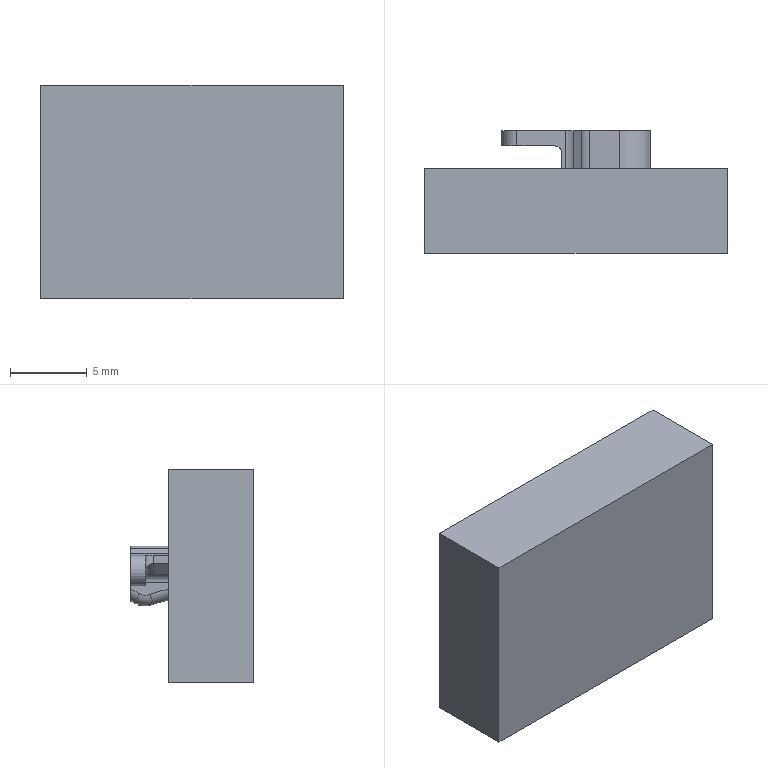NC program | NX | posted with a generic post | part box 19.7 x 8 x 13.91 mm
Lines 45 to 1140 of 12778:
(CAVITY_MILL_1 , TOOL : D4)
N76 T04 M6
N78 G54
N80 G17 G0 G90 X-8.599 Y7.638 B0. C0. S5500 M3
N82 G43 Z30. H4
N84 Z0.92
N86 G94 G1 Z-0.08 F1800.
N88 X-7.731 Y6.148
N90 G3 X-6.863 Y5.651 R1.
N92 G1 X-6.495 Y5.653
N94 X6.495
N96 X6.863 Y5.651
N98 G2 X7.047 Y5.469 R0.196
N100 G1 X7.048 Y5.107
N102 Y3.135
N104 X4.648
N106 G3 X2.923 Y3.103 R3.58
N108 G1 X0.887 Y2.557
N110 G2 X0.261 Y2.475 R2.42
N112 G1 X-1.249
N114 G3 X-1.796 Y3.253 R3.403
N116 G1 X-2.146 Y2.925
N118 G2 X-1.558 Y1.995 R2.923
N120 G1 X0.261
N122 G3 X1.012 Y2.094 R2.9
N124 G1 X3.048 Y2.639
N126 G2 X3.85 Y-3.455 R-3.1
N128 G1 X1.001
N130 X0.737 Y-3.613
N132 G2 X-0.858 Y-4.055 R3.1
N134 G1 X-2.85
N136 G2 X-6.95 Y0.045 R4.1
N138 G1 Y0.893
N140 G2 X-6.212 Y2.861 R3.007
N142 X-2.342 Y3.114 R2.731
N144 X-2.146 Y2.925 R2.923
N146 G1 X-1.796 Y3.253
N148 X4.648
N150 Y3.135
N152 X7.048
N154 Y1.254
N156 G2 X7.048 Y-1.964 R3.58
N158 G1 Y-5.107
N160 X7.047 Y-5.469
N162 G2 X6.863 Y-5.652 R0.196
N164 G1 X6.496 Y-5.653
N166 X-6.496
N168 X-6.863 Y-5.652
N170 G2 X-7.046 Y-5.469 R0.196
N172 G1 X-7.048 Y-5.107
N174 Y-1.787
N176 G2 X-7.43 Y0.045 R4.58
N178 G1 Y0.894
N180 G2 X-7.048 Y2.476 R3.487
N182 G1 Y5.107
N184 X-7.046 Y5.469
N186 G2 X-6.863 Y5.651 R0.195
N188 G3 X-6.027 Y6.201 R1.
N190 G1 X-4.995 Y8.253
N192 Z0.92
N194 G0 X-8.599 Y7.638 Z0.84
N196 G1 Z-0.16
N198 X-7.731 Y6.148
N200 G3 X-6.863 Y5.651 R1.
N202 G1 X-6.495 Y5.653
N204 X6.495
N206 X6.863 Y5.651
N208 G2 X7.047 Y5.469 R0.196
N210 G1 X7.048 Y5.107
N212 Y3.135
N214 X4.648
N216 G3 X2.923 Y3.103 R3.58
N218 G1 X0.887 Y2.557
N220 G2 X0.261 Y2.475 R2.42
N222 G1 X-1.228
N224 G3 X-1.755 Y3.253 R3.437
N226 G1 X-2.112 Y2.932
N228 G2 X-1.542 Y1.995 R2.957
N230 G1 X0.261
N232 G3 X1.012 Y2.094 R2.9
N234 G1 X3.048 Y2.639
N236 G2 X3.85 Y-3.455 R-3.1
N238 G1 X1.001
N240 X0.737 Y-3.613
N242 G2 X-0.858 Y-4.055 R3.1
N244 G1 X-2.85
N246 G2 X-6.95 Y0.045 R4.1
N248 G1 Y0.937
N250 G2 X-5.845 Y3.254 R2.971
N252 X-2.227 Y3.052 R2.73
N254 G1 X-2.112 Y2.932
N256 X-1.755 Y3.253
N258 X4.648
N260 Y3.135
N262 X7.048
N264 Y1.254
N266 G2 X7.048 Y-1.964 R3.58
N268 G1 Y-5.107
N270 X7.047 Y-5.469
N272 G2 X6.863 Y-5.652 R0.196
N274 G1 X6.496 Y-5.653
N276 X-6.496
N278 X-6.863 Y-5.652
N280 G2 X-7.046 Y-5.469 R0.196
N282 G1 X-7.048 Y-5.107
N284 Y-1.787
N286 G2 X-7.43 Y0.045 R4.58
N288 G1 Y0.937
N290 G2 X-7.048 Y2.521 R3.451
N292 G1 Y5.107
N294 X-7.046 Y5.469
N296 G2 X-6.863 Y5.651 R0.195
N298 G3 X-6.027 Y6.201 R1.
N300 G1 X-4.995 Y8.253
N302 Z0.84
N304 G0 X-8.599 Y7.638 Z0.76
N306 G1 Z-0.24
N308 X-7.731 Y6.148
N310 G3 X-6.863 Y5.651 R1.
N312 G1 X-6.495 Y5.653
N314 X6.495
N316 X6.863 Y5.651
N318 G2 X7.047 Y5.469 R0.196
N320 G1 X7.048 Y5.107
N322 Y3.135
N324 X4.648
N326 G3 X2.923 Y3.103 R3.58
N328 G1 X0.887 Y2.557
N330 G2 X0.261 Y2.475 R2.42
N332 G1 X-1.208
N334 G3 X-1.563 Y3.065 R3.543
N336 X-1.714 Y3.253 R3.224
N338 G1 X-2.077 Y2.938
N340 G2 X-1.948 Y2.779 R2.744
N342 X-1.527 Y1.995 R3.063
N344 G1 X0.261
N346 G3 X1.012 Y2.094 R2.9
N348 G1 X3.048 Y2.639
N350 G2 X3.85 Y-3.455 R-3.1
N352 G1 X1.001
N354 X0.737 Y-3.613
N356 G2 X-0.858 Y-4.055 R3.1
N358 G1 X-2.85
N360 G2 X-6.95 Y0.045 R4.1
N362 G1 Y0.981
N364 G2 X-6.22 Y2.94 R3.013
N366 X-2.077 Y2.938 R2.744
N368 G1 X-1.714 Y3.253
N370 X4.648
N372 Y3.135
N374 X7.048
N376 Y1.254
N378 G2 X7.048 Y-1.964 R3.58
N380 G1 Y-5.107
N382 X7.047 Y-5.469
N384 G2 X6.863 Y-5.652 R0.196
N386 G1 X6.496 Y-5.653
N388 X-6.496
N390 X-6.863 Y-5.652
N392 G2 X-7.046 Y-5.469 R0.196
N394 G1 X-7.048 Y-5.107
N396 Y-1.787
N398 G2 X-7.43 Y0.045 R4.58
N400 G1 Y0.982
N402 G2 X-7.048 Y2.563 R3.493
N404 G1 Y5.107
N406 X-7.046 Y5.469
N408 G2 X-6.863 Y5.651 R0.195
N410 G3 X-6.027 Y6.201 R1.
N412 G1 X-4.995 Y8.253
N414 Z0.76
N416 G0 X-8.599 Y7.638 Z0.68
N418 G1 Z-0.32
N420 X-7.731 Y6.148
N422 G3 X-6.863 Y5.652 R1.
N424 G1 X-6.495 Y5.653
N426 X6.495
N428 X6.863 Y5.652
N430 G2 X7.047 Y5.469 R0.196
N432 G1 X7.048 Y5.107
N434 Y3.135
N436 X4.648
N438 G3 X2.923 Y3.103 R3.58
N440 G1 X0.887 Y2.557
N442 G2 X0.261 Y2.475 R2.42
N444 G1 X-1.187
N446 G3 X-1.565 Y3.108 R3.414
N448 G1 X-1.68 Y3.253
N450 X-2.047 Y2.944
N452 X-1.948 Y2.82
N454 G2 X-1.512 Y1.995 R2.934
N456 G1 X0.261
N458 G3 X1.012 Y2.094 R2.9
N460 G1 X3.048 Y2.639
N462 G2 X3.85 Y-3.455 R-3.1
N464 G1 X1.001
N466 X0.737 Y-3.613
N468 G2 X-0.858 Y-4.055 R3.1
N470 G1 X-2.85
N472 G2 X-6.95 Y0.045 R4.1
N474 G1 Y1.025
N476 G2 X-6.402 Y2.751 R3.046
N478 X-2.047 Y2.944 R2.751
N480 G1 X-1.68 Y3.253
N482 X4.648
N484 Y3.135
N486 X7.048
N488 Y1.254
N490 G2 X7.048 Y-1.964 R3.58
N492 G1 Y-5.107
N494 X7.047 Y-5.469
N496 G2 X6.863 Y-5.652 R0.196
N498 G1 X6.496 Y-5.653
N500 X-6.496
N502 X-6.863 Y-5.652
N504 G2 X-7.046 Y-5.469 R0.196
N506 G1 X-7.048 Y-5.107
N508 Y-1.787
N510 G2 X-7.43 Y0.045 R4.58
N512 G1 Y1.027
N514 G2 X-7.048 Y2.605 R3.526
N516 G1 Y5.107
N518 X-7.046 Y5.469
N520 G2 X-6.863 Y5.652 R0.195
N522 G3 X-6.027 Y6.201 R1.
N524 G1 X-4.995 Y8.253
N526 Z0.68
N528 G0 X-8.599 Y7.638 Z0.6
N530 G1 Z-0.4
N532 X-7.731 Y6.148
N534 G3 X-6.863 Y5.652 R1.
N536 G1 X-6.495 Y5.653
N538 X6.495
N540 X6.863 Y5.652
N542 G2 X7.047 Y5.469 R0.196
N544 G1 X7.048 Y5.107
N546 Y3.135
N548 X4.648
N550 G3 X2.923 Y3.103 R3.58
N552 G1 X0.887 Y2.557
N554 G2 X0.261 Y2.475 R2.42
N556 G1 X-1.167
N558 G3 X-1.65 Y3.253 R3.354
N560 G1 X-2.019 Y2.947
N562 G2 X-1.497 Y1.995 R2.874
N564 G1 X0.261
N566 G3 X1.012 Y2.094 R2.9
N568 G1 X3.048 Y2.639
N570 G2 X3.85 Y-3.455 R-3.1
N572 G1 X1.001
N574 X0.737 Y-3.613
N576 G2 X-0.858 Y-4.055 R3.1
N578 G1 X-2.85
N580 G2 X-6.95 Y0.045 R4.1
N582 G1 Y1.069
N584 G2 X-6.286 Y2.94 R2.982
N586 X-2.227 Y3.171 R2.756
N588 X-2.019 Y2.947 R2.874
N590 G1 X-1.65 Y3.253
N592 X4.648
N594 Y3.135
N596 X7.048
N598 Y1.254
N600 G2 X7.048 Y-1.964 R3.58
N602 G1 Y-5.107
N604 X7.047 Y-5.469
N606 G2 X6.863 Y-5.652 R0.196
N608 G1 X6.496 Y-5.653
N610 X-6.496
N612 X-6.863 Y-5.652
N614 G2 X-7.046 Y-5.469 R0.196
N616 G1 X-7.048 Y-5.107
N618 Y-1.787
N620 G2 X-7.43 Y0.045 R4.58
N622 G1 Y1.069
N624 G2 X-7.048 Y2.645 R3.462
N626 G1 Y5.107
N628 X-7.046 Y5.469
N630 G2 X-6.863 Y5.652 R0.195
N632 G3 X-6.027 Y6.201 R1.
N634 G1 X-4.995 Y8.253
N636 Z0.6
N638 G0 X-8.599 Y7.638 Z0.52
N640 G1 Z-0.48
N642 X-7.731 Y6.148
N644 G3 X-6.863 Y5.652 R1.
N646 G1 X-6.495 Y5.653
N648 X6.495
N650 X6.863 Y5.652
N652 G2 X7.047 Y5.469 R0.196
N654 G1 X7.048 Y5.107
N656 Y3.135
N658 X4.648
N660 G3 X2.923 Y3.103 R3.58
N662 G1 X0.887 Y2.557
N664 G2 X0.261 Y2.475 R2.42
N666 G1 X-1.149
N668 G3 X-1.244 Y2.671 R2.683
N670 X-1.62 Y3.253 R3.252
N672 G1 X-1.993 Y2.951
N674 G2 X-1.67 Y2.449 R2.772
N676 X-1.487 Y1.995 R2.203
N678 G1 X0.261
N680 G3 X1.012 Y2.094 R2.9
N682 G1 X3.048 Y2.639
N684 G2 X3.85 Y-3.455 R-3.1
N686 G1 X1.001
N688 X0.737 Y-3.613
N690 G2 X-0.858 Y-4.055 R3.1
N692 G1 X-2.85
N694 G2 X-6.95 Y0.045 R4.1
N696 G1 Y1.112
N698 G2 X-6.402 Y2.823 R2.964
N700 X-1.993 Y2.951 R2.772
N702 G1 X-1.62 Y3.253
N704 X4.648
N706 Y3.135
N708 X7.048
N710 Y1.254
N712 G2 X7.048 Y-1.964 R3.58
N714 G1 Y-5.107
N716 X7.047 Y-5.469
N718 G2 X6.863 Y-5.652 R0.196
N720 G1 X6.496 Y-5.653
N722 X-6.496
N724 X-6.863 Y-5.652
N726 G2 X-7.046 Y-5.469 R0.196
N728 G1 X-7.048 Y-5.107
N730 Y-1.787
N732 G2 X-7.43 Y0.045 R4.58
N734 G1 Y1.113
N736 G2 X-7.048 Y2.683 R3.444
N738 G1 Y5.107
N740 X-7.046 Y5.469
N742 G2 X-6.863 Y5.652 R0.195
N744 G3 X-6.027 Y6.201 R1.
N746 G1 X-4.996 Y8.253
N748 Z0.52
N750 G0 X-8.599 Y7.638 Z0.44
N752 G1 Z-0.56
N754 X-7.731 Y6.148
N756 G3 X-6.863 Y5.652 R1.
N758 G1 X-6.495 Y5.653
N760 X6.495
N762 X6.863 Y5.652
N764 G2 X7.047 Y5.469 R0.196
N766 G1 X7.048 Y5.107
N768 Y3.135
N770 X4.648
N772 G3 X2.923 Y3.103 R3.58
N774 G1 X0.887 Y2.557
N776 G2 X0.261 Y2.475 R2.42
N778 G1 X-1.137
N780 G3 X-1.598 Y3.253 R3.265
N782 G1 X-1.973 Y2.954
N784 G2 X-1.476 Y1.995 R2.785
N786 G1 X0.261
N788 G3 X1.012 Y2.094 R2.9
N790 G1 X3.048 Y2.639
N792 G2 X3.85 Y-3.455 R-3.1
N794 G1 X1.001
N796 X0.737 Y-3.613
N798 G2 X-0.858 Y-4.055 R3.1
N800 G1 X-2.85
N802 G2 X-6.95 Y0.045 R4.1
N804 G1 Y1.156
N806 G2 X-6.402 Y2.854 R2.943
N808 X-1.973 Y2.954 R2.785
N810 G1 X-1.598 Y3.253
N812 X4.648
N814 Y3.135
N816 X7.048
N818 Y1.254
N820 G2 X7.048 Y-1.964 R3.58
N822 G1 Y-5.107
N824 X7.047 Y-5.469
N826 G2 X6.863 Y-5.652 R0.196
N828 G1 X6.496 Y-5.653
N830 X-6.496
N832 X-6.863 Y-5.652
N834 G2 X-7.046 Y-5.469 R0.196
N836 G1 X-7.048 Y-5.107
N838 Y-1.787
N840 G2 X-7.43 Y0.045 R4.58
N842 G1 Y1.158
N844 G2 X-7.048 Y2.715 R3.423
N846 G1 Y5.107
N848 X-7.046 Y5.469
N850 G2 X-6.863 Y5.652 R0.196
N852 G3 X-6.027 Y6.201 R1.
N854 G1 X-4.996 Y8.253
N856 Z0.44
N858 G0 X-8.599 Y7.638 Z0.36
N860 G1 Z-0.64
N862 X-7.731 Y6.148
N864 G3 X-6.863 Y5.652 R1.
N866 G1 X-6.495 Y5.653
N868 X6.495
N870 X6.863 Y5.652
N872 G2 X7.047 Y5.469 R0.196
N874 G1 X7.048 Y5.107
N876 Y3.135
N878 X4.648
N880 G3 X2.923 Y3.103 R3.58
N882 G1 X0.887 Y2.557
N884 G2 X0.261 Y2.475 R2.42
N886 G1 X-1.128
N888 G3 X-1.583 Y3.253 R3.269
N890 G1 X-1.96 Y2.956
N892 G2 X-1.469 Y1.995 R2.789
N894 G1 X0.261
N896 G3 X1.012 Y2.094 R2.9
N898 G1 X3.048 Y2.639
N900 G2 X3.85 Y-3.455 R-3.1
N902 G1 X1.001
N904 X0.737 Y-3.613
N906 G2 X-0.858 Y-4.055 R3.1
N908 G1 X-2.85
N910 G2 X-6.95 Y0.045 R4.1
N912 G1 Y1.195
N914 G2 X-5.845 Y3.446 R2.854
N916 X-1.96 Y2.956 R2.789
N918 G1 X-1.583 Y3.253
N920 X4.648
N922 Y3.135
N924 X7.048
N926 Y1.254
N928 G2 X7.048 Y-1.964 R3.58
N930 G1 Y-5.107
N932 X7.047 Y-5.469
N934 G2 X6.863 Y-5.652 R0.196
N936 G1 X6.496 Y-5.653
N938 X-6.496
N940 X-6.863 Y-5.652
N942 G2 X-7.046 Y-5.469 R0.196
N944 G1 X-7.048 Y-5.107
N946 Y-1.787
N948 G2 X-7.43 Y0.045 R4.58
N950 G1 Y1.195
N952 G2 X-7.048 Y2.741 R3.334
N954 G1 Y5.107
N956 X-7.046 Y5.469
N958 G2 X-6.863 Y5.652 R0.196
N960 G3 X-6.027 Y6.201 R1.
N962 G1 X-4.996 Y8.253
N964 Z0.36
N966 G0 X-8.599 Y7.638 Z0.28
N968 G1 Z-0.72
N970 X-7.731 Y6.148
N972 G3 X-6.863 Y5.652 R1.
N974 G1 X-6.495 Y5.653
N976 X6.495
N978 X6.863 Y5.652
N980 G2 X7.047 Y5.469 R0.196
N982 G1 X7.048 Y5.107
N984 Y3.135
N986 X4.648
N988 G3 X2.923 Y3.103 R3.58
N990 G1 X0.887 Y2.557
N992 G2 X0.261 Y2.475 R2.42
N994 G1 X-1.12
N996 G3 X-1.571 Y3.253 R3.275
N998 G1 X-1.949 Y2.958
N1000 G2 X-1.462 Y1.995 R2.795
N1002 G1 X0.261
N1004 G3 X1.012 Y2.094 R2.9
N1006 G1 X3.048 Y2.639
N1008 G2 X3.85 Y-3.455 R-3.1
N1010 G1 X1.001
N1012 X0.737 Y-3.613
N1014 G2 X-0.858 Y-4.055 R3.1
N1016 G1 X-2.85
N1018 G2 X-6.95 Y0.045 R4.1
N1020 G1 Y1.225
N1022 G2 X-5.793 Y3.501 R2.836
N1024 X-1.949 Y2.958 R2.795
N1026 G1 X-1.571 Y3.253
N1028 X4.648
N1030 Y3.135
N1032 X7.048
N1034 Y1.254
N1036 G2 X7.048 Y-1.964 R3.58
N1038 G1 Y-5.107
N1040 X7.047 Y-5.469
N1042 G2 X6.863 Y-5.652 R0.197
N1044 G1 X6.496 Y-5.653
N1046 X-6.496
N1048 X-6.863 Y-5.652
N1050 G2 X-7.046 Y-5.469 R0.196
N1052 G1 X-7.048 Y-5.107
N1054 Y-1.786
N1056 G2 X-7.43 Y0.045 R4.58
N1058 G1 Y1.226
N1060 G2 X-7.048 Y2.76 R3.316
N1062 G1 Y5.107
N1064 X-7.046 Y5.469
N1066 G2 X-6.863 Y5.652 R0.196
N1068 G3 X-6.027 Y6.201 R1.
N1070 G1 X-4.996 Y8.253
N1072 Z0.28
N1074 G0 X-8.599 Y7.639 Z0.2
N1076 G1 Z-0.8
N1078 X-7.731 Y6.148
N1080 G3 X-6.863 Y5.652 R1.
N1082 G1 X-6.495 Y5.653
N1084 X6.495
N1086 X6.863 Y5.652
N1088 G2 X7.047 Y5.469 R0.196
N1090 G1 X7.048 Y5.107
N1092 Y3.135
N1094 X4.648
N1096 G3 X2.923 Y3.103 R3.58
N1098 G1 X0.887 Y2.557
N1100 G2 X0.261 Y2.475 R2.42
N1102 G1 X-1.112
N1104 G3 X-1.56 Y3.253 R3.279
N1106 G1 X-1.939 Y2.959
N1108 G2 X-1.455 Y1.995 R2.799
N1110 G1 X0.261
N1112 G3 X1.012 Y2.094 R2.9
N1114 G1 X3.048 Y2.639
N1116 G2 X3.85 Y-3.455 R-3.1
N1118 G1 X1.001
N1120 X0.737 Y-3.613
N1122 G2 X-0.858 Y-4.055 R3.1
N1124 G1 X-2.85
N1126 G2 X-6.95 Y0.045 R4.1
N1128 G1 Y1.245
N1130 G2 X-1.939 Y2.959 R2.799
N1132 G1 X-1.56 Y3.253
N1134 X4.648
N1136 Y3.135
N1138 X7.048
N1140 Y1.254
N1142 G2 X7.048 Y-1.964 R3.58
N1144 G1 Y-5.107
N1146 X7.047 Y-5.469
N1148 G2 X6.863 Y-5.652 R0.197
N1150 G1 X6.496 Y-5.653
N1152 X-6.496
N1154 X-6.863 Y-5.652
N1156 G2 X-7.047 Y-5.469 R0.196
N1158 G1 X-7.048 Y-5.107
N1160 Y-1.786
N1162 G2 X-7.43 Y0.045 R4.58
N1164 G1 Y1.245
N1166 G2 X-7.048 Y2.78 R3.279
N1168 G1 Y5.107
N1170 X-7.047 Y5.469
N1172 G2 X-6.863 Y5.652 R0.196
N1174 G3 X-6.027 Y6.201 R1.
N1176 G1 X-4.996 Y8.253
N1178 Z0.2
N1180 G0 X-8.599 Y7.639 Z0.12
N1182 G1 Z-0.88
N1184 X-7.731 Y6.148
N1186 G3 X-6.863 Y5.652 R1.
N1188 G1 X-6.495 Y5.653
N1190 X6.495
N1192 X6.863 Y5.652
N1194 G2 X7.047 Y5.469 R0.196
N1196 G1 X7.048 Y5.107
N1198 Y3.135
N1200 X4.648
N1202 G3 X2.923 Y3.103 R3.58
N1204 G1 X0.887 Y2.557
N1206 G2 X0.261 Y2.475 R2.42
N1208 G1 X-1.111
N1210 G3 X-1.557 Y3.253 R3.278
N1212 G1 X-1.937 Y2.96
N1214 G2 X-1.455 Y1.995 R2.798
N1216 G1 X0.261
N1218 G3 X1.012 Y2.094 R2.9
N1220 G1 X3.048 Y2.639
N1222 G2 X3.85 Y-3.455 R-3.1
N1224 G1 X1.001
N1226 X0.737 Y-3.613
N1228 G2 X-0.858 Y-4.055 R3.1
N1230 G1 X-2.85
N1232 G2 X-6.95 Y0.045 R4.1
N1234 G1 Y1.256
N1236 G2 X-1.937 Y2.96 R2.798
N1238 G1 X-1.557 Y3.253
N1240 X4.648
N1242 Y3.135
N1244 X7.048
N1246 Y1.254
N1248 G2 X7.048 Y-1.964 R3.58
N1250 G1 Y-5.107
N1252 X7.047 Y-5.469
N1254 G2 X6.863 Y-5.652 R0.197
N1256 G1 X6.496 Y-5.653
N1258 X-6.496
N1260 X-6.863 Y-5.652
N1262 G2 X-7.047 Y-5.469 R0.196
N1264 G1 X-7.048 Y-5.107
N1266 Y-1.786
N1268 G2 X-7.43 Y0.045 R4.58
N1270 G1 Y1.257
N1272 G2 X-7.048 Y2.786 R3.278
N1274 G1 Y5.107
N1276 X-7.047 Y5.469
N1278 G2 X-6.863 Y5.652 R0.196
N1280 G3 X-6.027 Y6.201 R1.
N1282 G1 X-4.996 Y8.253
N1284 Z0.12
N1286 G0 X-8.599 Y7.639 Z0.04
N1288 G1 Z-0.96
N1290 X-7.731 Y6.148
N1292 G3 X-6.863 Y5.652 R1.
N1294 G1 X-6.495 Y5.653
N1296 X6.495
N1298 X6.863 Y5.652
N1300 G2 X7.047 Y5.469 R0.196
N1302 G1 X7.048 Y5.107
N1304 Y3.135
N1306 X4.648
N1308 G3 X2.923 Y3.103 R3.58
N1310 G1 X0.887 Y2.557
N1312 G2 X0.261 Y2.475 R2.42
N1314 G1 X-1.111
N1316 G3 X-1.557 Y3.253 R3.278
N1318 G1 X-1.937 Y2.96
N1320 G2 X-1.455 Y1.995 R2.798
N1322 G1 X0.261
N1324 G3 X1.012 Y2.094 R2.9
N1326 G1 X3.048 Y2.639
N1328 G2 X3.85 Y-3.455 R-3.1
N1330 G1 X1.001
N1332 X0.737 Y-3.613
N1334 G2 X-0.858 Y-4.055 R3.1
N1336 G1 X-2.85
N1338 G2 X-6.95 Y0.045 R4.1
N1340 G1 Y1.259
N1342 G2 X-1.937 Y2.96 R2.798
N1344 G1 X-1.557 Y3.253
N1346 X4.648
N1348 Y3.135
N1350 X7.048
N1352 Y1.254
N1354 G2 X7.048 Y-1.964 R3.58
N1356 G1 Y-5.107
N1358 X7.047 Y-5.469
N1360 G2 X6.863 Y-5.652 R0.197
N1362 G1 X6.496 Y-5.653
N1364 X-6.496
N1366 X-6.863 Y-5.652
N1368 G2 X-7.047 Y-5.469 R0.196
N1370 G1 X-7.048 Y-5.107
N1372 Y-1.786
N1374 G2 X-7.43 Y0.045 R4.58
N1376 G1 Y1.261
N1378 G2 X-7.048 Y2.786 R3.278
N1380 G1 Y5.107
N1382 X-7.047 Y5.469
N1384 G2 X-6.863 Y5.652 R0.196
N1386 G3 X-6.027 Y6.201 R1.
N1388 G1 X-4.996 Y8.253
N1390 Z0.04
N1392 G0 X-8.599 Y7.639 Z-0.04
N1394 G1 Z-1.04
N1396 X-7.731 Y6.148
N1398 G3 X-6.863 Y5.652 R1.
N1400 G1 X-6.495 Y5.653
N1402 X6.495
N1404 X6.863 Y5.652
N1406 G2 X7.047 Y5.469 R0.196
N1408 G1 X7.048 Y5.107
N1410 Y3.135
N1412 X4.648
N1414 G3 X2.923 Y3.103 R3.58
N1416 G1 X0.887 Y2.557
N1418 G2 X0.261 Y2.475 R2.42
N1420 G1 X-1.111
N1422 G3 X-1.557 Y3.253 R3.278
N1424 G1 X-1.937 Y2.96
N1426 G2 X-1.454 Y1.995 R2.798
N1428 G1 X0.261
N1430 G3 X1.012 Y2.094 R2.9
N1432 G1 X3.048 Y2.639
N1434 G2 X3.85 Y-3.455 R-3.1
N1436 G1 X1.001
N1438 X0.737 Y-3.613
N1440 G2 X-0.858 Y-4.055 R3.1
N1442 G1 X-2.85
N1444 G2 X-6.95 Y0.045 R4.1
N1446 G1 Y1.252
N1448 G2 X-1.937 Y2.96 R2.798
N1450 G1 X-1.557 Y3.253
N1452 X4.648
N1454 Y3.135
N1456 X7.048
N1458 Y1.254
N1460 G2 X7.048 Y-1.964 R3.58
N1462 G1 Y-5.107
N1464 X7.047 Y-5.469
N1466 G2 X6.863 Y-5.652 R0.197
N1468 G1 X6.496 Y-5.653
N1470 X-6.496
N1472 X-6.863 Y-5.652
N1474 G2 X-7.047 Y-5.469 R0.196
N1476 G1 X-7.048 Y-5.107
N1478 Y-1.786
N1480 G2 X-7.43 Y0.045 R4.58
N1482 G1 Y1.252
N1484 G2 X-7.048 Y2.785 R3.278
N1486 G1 Y5.107
N1488 X-7.047 Y5.469
N1490 G2 X-6.863 Y5.652 R0.196
N1492 G3 X-6.027 Y6.201 R1.
N1494 G1 X-4.996 Y8.253
N1496 Z-0.04
N1498 G0 X-8.599 Y7.639 Z-0.12
N1500 G1 Z-1.12
N1502 X-7.731 Y6.148
N1504 G3 X-6.863 Y5.652 R1.
N1506 G1 X-6.495 Y5.653
N1508 X6.495
N1510 X6.863 Y5.652
N1512 G2 X7.047 Y5.469 R0.196
N1514 G1 X7.048 Y5.107
N1516 Y3.135
N1518 X4.648
N1520 G3 X2.923 Y3.103 R3.58
N1522 G1 X0.887 Y2.557
N1524 G2 X0.261 Y2.475 R2.42
N1526 G1 X-1.111
N1528 G3 X-1.557 Y3.253 R3.278
N1530 G1 X-1.937 Y2.96
N1532 G2 X-1.454 Y1.995 R2.798
N1534 G1 X0.261
N1536 G3 X1.012 Y2.094 R2.9
N1538 G1 X3.048 Y2.639
N1540 G2 X3.85 Y-3.455 R-3.1
N1542 G1 X1.001
N1544 X0.737 Y-3.613
N1546 G2 X-0.858 Y-4.055 R3.1
N1548 G1 X-2.85
N1550 G2 X-6.95 Y0.045 R4.1
N1552 G1 Y1.252
N1554 G2 X-1.937 Y2.96 R2.798
N1556 G1 X-1.557 Y3.253
N1558 X4.648
N1560 Y3.135
N1562 X7.048
N1564 Y1.254
N1566 G2 X7.048 Y-1.964 R3.58
N1568 G1 Y-5.107
N1570 X7.047 Y-5.469
N1572 G2 X6.863 Y-5.652 R0.197
N1574 G1 X6.496 Y-5.653
N1576 X-6.496
N1578 X-6.863 Y-5.652
N1580 G2 X-7.047 Y-5.469 R0.196
N1582 G1 X-7.048 Y-5.107
N1584 Y-1.786
N1586 G2 X-7.43 Y0.045 R4.58
N1588 G1 Y1.253
N1590 G2 X-7.048 Y2.785 R3.278
N1592 G1 Y5.107
N1594 X-7.047 Y5.469
N1596 G2 X-6.863 Y5.652 R0.196
N1598 G3 X-6.027 Y6.201 R1.
N1600 G1 X-4.996 Y8.253
N1602 Z-0.12
N1604 G0 X-8.599 Y7.639 Z-0.2
N1606 G1 Z-1.2
N1608 X-7.731 Y6.148
N1610 G3 X-6.863 Y5.652 R1.
N1612 G1 X-6.495 Y5.653
N1614 X6.495
N1616 X6.863 Y5.652
N1618 G2 X7.047 Y5.469 R0.196
N1620 G1 X7.048 Y5.107
N1622 Y3.135
N1624 X4.648
N1626 G3 X2.923 Y3.103 R3.58
N1628 G1 X0.887 Y2.557
N1630 G2 X0.261 Y2.475 R2.42
N1632 G1 X-1.111
N1634 G3 X-1.556 Y3.253 R3.279
N1636 G1 X-1.936 Y2.96
N1638 G2 X-1.454 Y1.995 R2.799
N1640 G1 X0.261
N1642 G3 X1.012 Y2.094 R2.9
N1644 G1 X3.048 Y2.639
N1646 G2 X3.85 Y-3.455 R-3.1
N1648 G1 X1.001
N1650 X0.737 Y-3.613
N1652 G2 X-0.858 Y-4.055 R3.1
N1654 G1 X-2.85
N1656 G2 X-6.95 Y0.045 R4.1
N1658 G1 Y1.252
N1660 G2 X-1.936 Y2.96 R2.799
N1662 G1 X-1.556 Y3.253
N1664 X4.648
N1666 Y3.135
N1668 X7.048
N1670 Y1.253
N1672 G2 X7.048 Y-1.964 R3.58
N1674 G1 Y-5.107
N1676 X7.047 Y-5.469
N1678 G2 X6.863 Y-5.652 R0.197
N1680 G1 X6.496 Y-5.653
N1682 X-6.496
N1684 X-6.863 Y-5.652
N1686 G2 X-7.047 Y-5.469 R0.196
N1688 G1 X-7.048 Y-5.107
N1690 Y-1.786
N1692 G2 X-7.43 Y0.045 R4.58
N1694 G1 Y1.253
N1696 G2 X-7.048 Y2.785 R3.279
N1698 G1 Y5.107
N1700 X-7.047 Y5.469
N1702 G2 X-6.863 Y5.652 R0.196
N1704 G3 X-6.027 Y6.201 R1.
N1706 G1 X-4.996 Y8.253
N1708 Z-0.2
N1710 G0 X-8.599 Y7.639 Z-0.28
N1712 G1 Z-1.28
N1714 X-7.731 Y6.148
N1716 G3 X-6.863 Y5.652 R1.
N1718 G1 X-6.495 Y5.653
N1720 X6.495
N1722 X6.863 Y5.652
N1724 G2 X7.047 Y5.469 R0.196
N1726 G1 X7.048 Y5.107
N1728 Y3.135
N1730 X4.648
N1732 G3 X2.923 Y3.103 R3.58
N1734 G1 X0.887 Y2.557
N1736 G2 X0.261 Y2.475 R2.42
N1738 G1 X-1.11
N1740 G3 X-1.556 Y3.253 R3.279
N1742 G1 X-1.936 Y2.96
N1744 G2 X-1.454 Y1.995 R2.799
N1746 G1 X0.261
N1748 G3 X1.012 Y2.094 R2.9
N1750 G1 X3.048 Y2.639
N1752 G2 X3.85 Y-3.455 R-3.1
N1754 G1 X1.001
N1756 X0.737 Y-3.613
N1758 G2 X-0.858 Y-4.055 R3.1
N1760 G1 X-2.85
N1762 G2 X-6.95 Y0.045 R4.1
N1764 G1 Y1.252
N1766 G2 X-1.936 Y2.96 R2.799
N1768 G1 X-1.556 Y3.253
N1770 X4.648
N1772 Y3.135
N1774 X7.048
N1776 Y1.253
N1778 G2 X7.048 Y-1.964 R3.58
N1780 G1 Y-5.107
N1782 X7.047 Y-5.469
N1784 G2 X6.863 Y-5.652 R0.197
N1786 G1 X6.496 Y-5.653
N1788 X-6.496
N1790 X-6.863 Y-5.652
N1792 G2 X-7.047 Y-5.469 R0.197
N1794 G1 X-7.048 Y-5.107
N1796 Y-1.786
N1798 G2 X-7.43 Y0.045 R4.58
N1800 G1 Y1.253
N1802 G2 X-7.048 Y2.785 R3.279
N1804 G1 Y5.107
N1806 X-7.047 Y5.469
N1808 G2 X-6.863 Y5.652 R0.196
N1810 G3 X-6.027 Y6.201 R1.
N1812 G1 X-4.996 Y8.253
N1814 Z-0.28
N1816 G0 X-8.599 Y7.639 Z-0.36
N1818 G1 Z-1.36
N1820 X-7.731 Y6.148
N1822 G3 X-6.863 Y5.652 R1.
N1824 G1 X-6.495 Y5.653
N1826 X6.495
N1828 X6.863 Y5.652
N1830 G2 X7.047 Y5.469 R0.197
N1832 G1 X7.048 Y5.108
N1834 Y3.135
N1836 X4.648
N1838 G3 X2.923 Y3.103 R3.58
N1840 G1 X0.887 Y2.557
N1842 G2 X0.261 Y2.475 R2.42
N1844 G1 X-1.11
N1846 G3 X-1.556 Y3.253 R3.279
N1848 G1 X-1.936 Y2.96
N1850 G2 X-1.454 Y1.995 R2.799
N1852 G1 X0.261
N1854 G3 X1.012 Y2.094 R2.9
N1856 G1 X3.048 Y2.639
N1858 G2 X3.85 Y-3.455 R-3.1
N1860 G1 X1.001
N1862 X0.737 Y-3.613
N1864 G2 X-0.858 Y-4.055 R3.1
N1866 G1 X-2.85
N1868 G2 X-6.95 Y0.045 R4.1
N1870 G1 Y1.252
N1872 G2 X-1.936 Y2.96 R2.799
N1874 G1 X-1.556 Y3.253
N1876 X4.648
N1878 Y3.135
N1880 X7.048
N1882 Y1.253
N1884 G2 X7.048 Y-1.964 R3.58
N1886 G1 Y-5.108
N1888 X7.047 Y-5.469
N1890 G2 X6.862 Y-5.652 R0.197
N1892 G1 X6.496 Y-5.653
N1894 X-6.496
N1896 X-6.863 Y-5.652
N1898 G2 X-7.047 Y-5.469 R0.197
N1900 G1 X-7.048 Y-5.107
N1902 Y-1.786
N1904 G2 X-7.43 Y0.045 R4.58
N1906 G1 Y1.253
N1908 G2 X-7.048 Y2.785 R3.279
N1910 G1 Y5.107
N1912 X-7.047 Y5.469
N1914 G2 X-6.863 Y5.652 R0.196
N1916 G3 X-6.027 Y6.201 R1.
N1918 G1 X-4.996 Y8.253
N1920 Z-0.36
N1922 G0 X-8.599 Y7.639 Z-0.44
N1924 G1 Z-1.44
N1926 X-7.731 Y6.148
N1928 G3 X-6.863 Y5.652 R1.
N1930 G1 X-6.495 Y5.653
N1932 X6.495
N1934 X6.863 Y5.652
N1936 G2 X7.047 Y5.469 R0.197
N1938 G1 X7.048 Y5.108
N1940 Y3.135
N1942 X4.648
N1944 G3 X2.923 Y3.103 R3.58
N1946 G1 X0.887 Y2.557
N1948 G2 X0.261 Y2.475 R2.42
N1950 G1 X-1.11
N1952 G3 X-1.556 Y3.253 R3.279
N1954 G1 X-1.936 Y2.96
N1956 G2 X-1.453 Y1.995 R2.799
N1958 G1 X0.261
N1960 G3 X1.012 Y2.094 R2.9
N1962 G1 X3.048 Y2.639
N1964 G2 X3.85 Y-3.455 R-3.1
N1966 G1 X1.001
N1968 X0.737 Y-3.613
N1970 G2 X-0.858 Y-4.055 R3.1
N1972 G1 X-2.85
N1974 G2 X-6.95 Y0.045 R4.1
N1976 G1 Y1.252
N1978 G2 X-1.936 Y2.96 R2.799
N1980 G1 X-1.556 Y3.253
N1982 X4.648
N1984 Y3.135
N1986 X7.048
N1988 Y1.253
N1990 G2 X7.048 Y-1.963 R3.58
N1992 G1 Y-5.108
N1994 X7.047 Y-5.469
N1996 G2 X6.862 Y-5.652 R0.197
N1998 G1 X6.496 Y-5.653
N2000 X-6.496
N2002 X-6.863 Y-5.652
N2004 G2 X-7.047 Y-5.469 R0.197
N2006 G1 X-7.048 Y-5.107
N2008 Y-1.786
N2010 G2 X-7.43 Y0.045 R4.58
N2012 G1 Y1.253
N2014 G2 X-7.048 Y2.785 R3.279
N2016 G1 Y5.107
N2018 X-7.047 Y5.469
N2020 G2 X-6.863 Y5.652 R0.196
N2022 G3 X-6.027 Y6.201 R1.
N2024 G1 X-4.996 Y8.253
N2026 Z-0.44
N2028 G0 X-8.599 Y7.639 Z-0.52
N2030 G1 Z-1.52
N2032 X-7.731 Y6.148
N2034 G3 X-6.863 Y5.652 R1.
N2036 G1 X-6.495 Y5.653
N2038 X6.495
N2040 X6.863 Y5.652
N2042 G2 X7.047 Y5.469 R0.197
N2044 G1 X7.048 Y5.108
N2046 Y3.135
N2048 X4.648
N2050 G3 X2.923 Y3.103 R3.58
N2052 G1 X0.887 Y2.557
N2054 G2 X0.261 Y2.475 R2.42
N2056 G1 X-1.11
N2058 G3 X-1.556 Y3.253 R3.279
N2060 G1 X-1.936 Y2.96
N2062 G2 X-1.453 Y1.995 R2.799
N2064 G1 X0.261
N2066 G3 X1.012 Y2.094 R2.9
N2068 G1 X3.048 Y2.639
N2070 G2 X3.85 Y-3.455 R-3.1
N2072 G1 X1.001
N2074 X0.737 Y-3.613
N2076 G2 X-0.858 Y-4.055 R3.1
N2078 G1 X-2.85
N2080 G2 X-6.95 Y0.045 R4.1
N2082 G1 Y1.252
N2084 G2 X-1.936 Y2.96 R2.799
N2086 G1 X-1.556 Y3.253
N2088 X4.648
N2090 Y3.135
N2092 X7.048
N2094 Y1.253
N2096 G2 X7.048 Y-1.963 R3.58
N2098 G1 Y-5.108
N2100 X7.047 Y-5.469
N2102 G2 X6.862 Y-5.652 R0.197
N2104 G1 X6.496 Y-5.653
N2106 X-6.496
N2108 X-6.862 Y-5.652
N2110 G2 X-7.047 Y-5.469 R0.197
N2112 G1 X-7.048 Y-5.107
N2114 Y-1.786
N2116 G2 X-7.43 Y0.045 R4.58
N2118 G1 Y1.253
N2120 G2 X-7.048 Y2.785 R3.279
N2122 G1 Y5.107
N2124 X-7.047 Y5.469
N2126 G2 X-6.863 Y5.652 R0.196
N2128 G3 X-6.027 Y6.201 R1.
N2130 G1 X-4.996 Y8.253
N2132 Z-0.52
N2134 G0 X-8.599 Y7.639 Z-0.6
N2136 G1 Z-1.6
N2138 X-7.731 Y6.148
N2140 G3 X-6.863 Y5.652 R1.
N2142 G1 X-6.495 Y5.653
N2144 X6.495
N2146 X6.863 Y5.652
N2148 G2 X7.047 Y5.469 R0.197
N2150 G1 X7.048 Y5.108
N2152 Y3.135
N2154 X4.648
N2156 G3 X2.923 Y3.103 R3.58
N2158 G1 X0.887 Y2.557
N2160 G2 X0.261 Y2.475 R2.42
N2162 G1 X-1.109
N2164 G3 X-1.556 Y3.253 R3.279
N2166 G1 X-1.935 Y2.96
N2168 G2 X-1.453 Y1.995 R2.799
N2170 G1 X0.261
N2172 G3 X1.012 Y2.094 R2.9
N2174 G1 X3.048 Y2.639
N2176 G2 X3.85 Y-3.455 R-3.1
N2178 G1 X1.001
N2180 X0.737 Y-3.613
N2182 G2 X-0.858 Y-4.055 R3.1
N2184 G1 X-2.85
N2186 G2 X-6.95 Y0.045 R4.1
N2188 G1 Y1.252
N2190 G2 X-1.935 Y2.96 R2.799
N2192 G1 X-1.556 Y3.253
N2194 X4.648
N2196 Y3.135
N2198 X7.048
N2200 Y1.253
N2202 G2 X7.048 Y-1.963 R3.58
N2204 G1 Y-5.108
N2206 X7.047 Y-5.469
N2208 G2 X6.862 Y-5.652 R0.197
N2210 G1 X6.496 Y-5.654
N2212 X-6.496
N2214 X-6.862 Y-5.652
N2216 G2 X-7.047 Y-5.469 R0.197
N2218 G1 X-7.048 Y-5.107
N2220 Y-1.786
N2222 G2 X-7.43 Y0.045 R4.58
N2224 G1 Y1.253
N2226 G2 X-7.048 Y2.785 R3.279
N2228 G1 Y5.107
N2230 X-7.047 Y5.469
N2232 G2 X-6.863 Y5.652 R0.196
N2234 G3 X-6.027 Y6.201 R1.
N2236 G1 X-4.996 Y8.253
N2238 Z-0.6
N2240 G0 X-8.599 Y7.639 Z-0.68
N2242 G1 Z-1.68
N2244 X-7.731 Y6.148
N2246 G3 X-6.863 Y5.652 R1.
N2248 G1 X-6.495 Y5.653
N2250 X6.495
N2252 X6.863 Y5.652
N2254 G2 X7.047 Y5.469 R0.197
N2256 G1 X7.048 Y5.108
N2258 Y3.135
N2260 X4.648